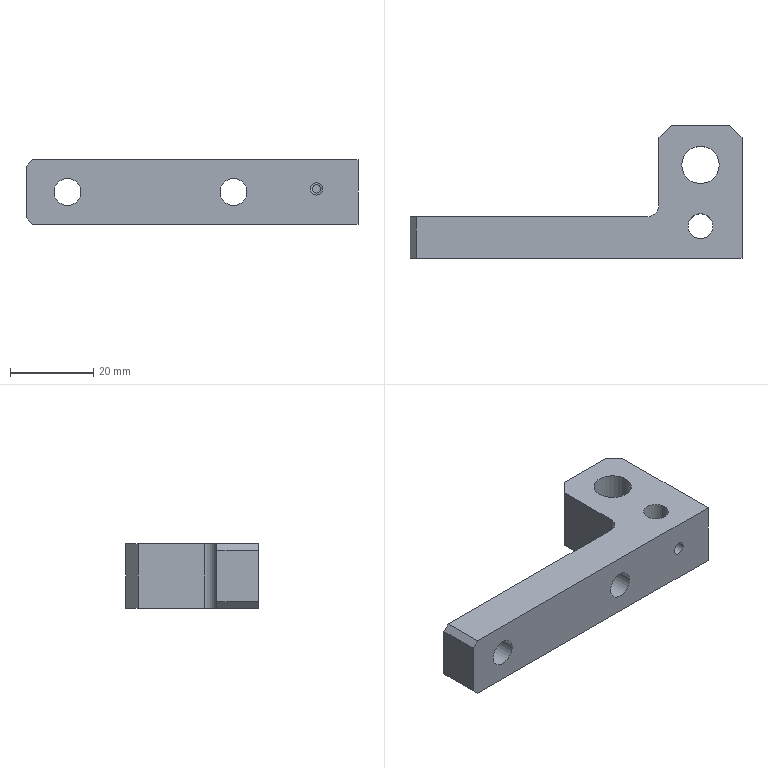NC program | NX | posted with a generic post | part box 80 x 32 x 15.5 mm
Lines 3921 to 4741 of 7013:
(PLANAR_MILL_5 , TOOL : D4-12-D4-50-3T-FINISH)
N7792 T11 M6
N7794 G53
N7796 G17 G0 G90 X26.347 Y-4.914 B0. C0. S3000 M3
N7798 G43 Z20. H11
N7800 Z0.5
N7802 G94 G1 X26.264 Y-5.105 Z0.499 F200.
N7804 X26.137 Y-5.509 Z0.497
N7806 X26.054 Y-5.924 Z0.494
N7808 X26.015 Y-6.345 Z0.492
N7810 Y-6.655 Z0.491
N7812 X26.054 Y-7.076 Z0.488
N7814 X26.137 Y-7.491 Z0.486
N7816 X26.264 Y-7.895 Z0.484
N7818 X26.433 Y-8.283 Z0.482
N7820 X26.641 Y-8.65 Z0.48
N7822 X26.888 Y-8.994 Z0.477
N7824 X27.17 Y-9.31 Z0.475
N7826 X27.484 Y-9.594 Z0.473
N7828 X27.826 Y-9.843 Z0.471
N7830 X28.192 Y-10.055 Z0.468
N7832 X28.579 Y-10.226 Z0.466
N7834 X28.982 Y-10.356 Z0.464
N7836 X29.396 Y-10.442 Z0.462
N7838 X29.817 Y-10.484 Z0.46
N7840 X30.24 Y-10.481 Z0.457
N7842 X30.66 Y-10.433 Z0.455
N7844 X31.073 Y-10.341 Z0.453
N7846 X31.474 Y-10.205 Z0.451
N7848 X31.859 Y-10.028 Z0.449
N7850 X32.126 Y-9.874 Z0.447
N7852 X32.477 Y-9.626 Z0.445
N7854 X32.799 Y-9.341 Z0.442
N7856 X33.088 Y-9.024 Z0.44
N7858 X33.341 Y-8.677 Z0.438
N7860 X33.556 Y-8.305 Z0.436
N7862 X33.73 Y-7.912 Z0.433
N7864 X33.86 Y-7.503 Z0.431
N7866 X33.945 Y-7.082 Z0.429
N7868 X33.985 Y-6.655 Z0.427
N7870 Y-6.345 Z0.425
N7872 X33.945 Y-5.918 Z0.423
N7874 X33.86 Y-5.497 Z0.421
N7876 X33.73 Y-5.088 Z0.418
N7878 X33.556 Y-4.695 Z0.416
N7880 X33.341 Y-4.323 Z0.414
N7882 X33.088 Y-3.976 Z0.412
N7884 X32.799 Y-3.659 Z0.409
N7886 X32.477 Y-3.374 Z0.407
N7888 X32.126 Y-3.126 Z0.405
N7890 X31.859 Y-2.972 Z0.403
N7892 X31.474 Y-2.795 Z0.401
N7894 X31.073 Y-2.659 Z0.399
N7896 X30.66 Y-2.567 Z0.397
N7898 X30.24 Y-2.519 Z0.394
N7900 X29.817 Y-2.516 Z0.392
N7902 X29.396 Y-2.558 Z0.39
N7904 X28.982 Y-2.644 Z0.388
N7906 X28.579 Y-2.774 Z0.385
N7908 X28.192 Y-2.945 Z0.383
N7910 X27.826 Y-3.157 Z0.381
N7912 X27.484 Y-3.406 Z0.379
N7914 X27.17 Y-3.69 Z0.377
N7916 X26.888 Y-4.006 Z0.374
N7918 X26.641 Y-4.35 Z0.372
N7920 X26.433 Y-4.717 Z0.37
N7922 X26.264 Y-5.105 Z0.368
N7924 X26.137 Y-5.509 Z0.366
N7926 X26.054 Y-5.924 Z0.363
N7928 X26.015 Y-6.345 Z0.361
N7930 Y-6.655 Z0.36
N7932 X26.054 Y-7.076 Z0.357
N7934 X26.137 Y-7.491 Z0.355
N7936 X26.264 Y-7.895 Z0.353
N7938 X26.433 Y-8.283 Z0.351
N7940 X26.641 Y-8.65 Z0.348
N7942 X26.888 Y-8.994 Z0.346
N7944 X27.17 Y-9.31 Z0.344
N7946 X27.484 Y-9.594 Z0.342
N7948 X27.826 Y-9.843 Z0.34
N7950 X28.192 Y-10.055 Z0.337
N7952 X28.579 Y-10.226 Z0.335
N7954 X28.982 Y-10.356 Z0.333
N7956 X29.396 Y-10.442 Z0.331
N7958 X29.817 Y-10.484 Z0.328
N7960 X30.24 Y-10.481 Z0.326
N7962 X30.66 Y-10.433 Z0.324
N7964 X31.073 Y-10.341 Z0.322
N7966 X31.474 Y-10.205 Z0.32
N7968 X31.859 Y-10.028 Z0.317
N7970 X32.126 Y-9.874 Z0.316
N7972 X32.477 Y-9.626 Z0.314
N7974 X32.799 Y-9.341 Z0.311
N7976 X33.088 Y-9.024 Z0.309
N7978 X33.341 Y-8.677 Z0.307
N7980 X33.556 Y-8.305 Z0.305
N7982 X33.73 Y-7.912 Z0.302
N7984 X33.86 Y-7.503 Z0.3
N7986 X33.945 Y-7.082 Z0.298
N7988 X33.985 Y-6.655 Z0.296
N7990 Y-6.345 Z0.294
N7992 X33.945 Y-5.918 Z0.292
N7994 X33.86 Y-5.497 Z0.289
N7996 X33.73 Y-5.088 Z0.287
N7998 X33.556 Y-4.695 Z0.285
N8000 X33.341 Y-4.323 Z0.283
N8002 X33.088 Y-3.976 Z0.28
N8004 X32.799 Y-3.659 Z0.278
N8006 X32.477 Y-3.374 Z0.276
N8008 X32.126 Y-3.126 Z0.274
N8010 X31.859 Y-2.972 Z0.272
N8012 X31.474 Y-2.795 Z0.27
N8014 X31.073 Y-2.659 Z0.268
N8016 X30.66 Y-2.567 Z0.265
N8018 X30.24 Y-2.519 Z0.263
N8020 X29.817 Y-2.516 Z0.261
N8022 X29.396 Y-2.558 Z0.259
N8024 X28.982 Y-2.644 Z0.257
N8026 X28.579 Y-2.774 Z0.254
N8028 X28.192 Y-2.945 Z0.252
N8030 X27.826 Y-3.157 Z0.25
N8032 X27.484 Y-3.406 Z0.248
N8034 X27.17 Y-3.69 Z0.245
N8036 X26.888 Y-4.006 Z0.243
N8038 X26.641 Y-4.35 Z0.241
N8040 X26.433 Y-4.717 Z0.239
N8042 X26.264 Y-5.105 Z0.237
N8044 X26.137 Y-5.509 Z0.234
N8046 X26.054 Y-5.924 Z0.232
N8048 X26.015 Y-6.345 Z0.23
N8050 Y-6.655 Z0.228
N8052 X26.054 Y-7.076 Z0.226
N8054 X26.137 Y-7.491 Z0.224
N8056 X26.264 Y-7.895 Z0.222
N8058 X26.433 Y-8.283 Z0.219
N8060 X26.641 Y-8.65 Z0.217
N8062 X26.888 Y-8.994 Z0.215
N8064 X27.17 Y-9.31 Z0.213
N8066 X27.484 Y-9.594 Z0.211
N8068 X27.826 Y-9.843 Z0.208
N8070 X28.192 Y-10.055 Z0.206
N8072 X28.579 Y-10.226 Z0.204
N8074 X28.982 Y-10.356 Z0.202
N8076 X29.396 Y-10.442 Z0.2
N8078 X29.817 Y-10.484 Z0.197
N8080 X30.24 Y-10.481 Z0.195
N8082 X30.66 Y-10.433 Z0.193
N8084 X31.073 Y-10.341 Z0.191
N8086 X31.474 Y-10.205 Z0.188
N8088 X31.859 Y-10.028 Z0.186
N8090 X32.126 Y-9.874 Z0.185
N8092 X32.477 Y-9.626 Z0.182
N8094 X32.799 Y-9.341 Z0.18
N8096 X33.088 Y-9.024 Z0.178
N8098 X33.341 Y-8.677 Z0.176
N8100 X33.556 Y-8.305 Z0.173
N8102 X33.73 Y-7.912 Z0.171
N8104 X33.86 Y-7.503 Z0.169
N8106 X33.945 Y-7.082 Z0.167
N8108 X33.985 Y-6.655 Z0.164
N8110 Y-6.345 Z0.163
N8112 X33.945 Y-5.918 Z0.161
N8114 X33.86 Y-5.497 Z0.158
N8116 X33.73 Y-5.088 Z0.156
N8118 X33.556 Y-4.695 Z0.154
N8120 X33.341 Y-4.323 Z0.152
N8122 X33.088 Y-3.976 Z0.149
N8124 X32.799 Y-3.659 Z0.147
N8126 X32.477 Y-3.374 Z0.145
N8128 X32.126 Y-3.126 Z0.143
N8130 X31.859 Y-2.972 Z0.141
N8132 X31.474 Y-2.795 Z0.139
N8134 X31.073 Y-2.659 Z0.137
N8136 X30.66 Y-2.567 Z0.134
N8138 X30.24 Y-2.519 Z0.132
N8140 X29.817 Y-2.516 Z0.13
N8142 X29.396 Y-2.558 Z0.128
N8144 X28.982 Y-2.644 Z0.125
N8146 X28.579 Y-2.774 Z0.123
N8148 X28.192 Y-2.945 Z0.121
N8150 X27.826 Y-3.157 Z0.119
N8152 X27.484 Y-3.406 Z0.117
N8154 X27.17 Y-3.69 Z0.114
N8156 X26.888 Y-4.006 Z0.112
N8158 X26.641 Y-4.35 Z0.11
N8160 X26.433 Y-4.717 Z0.108
N8162 X26.264 Y-5.105 Z0.105
N8164 X26.137 Y-5.509 Z0.103
N8166 X26.054 Y-5.924 Z0.101
N8168 X26.015 Y-6.345 Z0.099
N8170 Y-6.655 Z0.097
N8172 X26.054 Y-7.076 Z0.095
N8174 X26.137 Y-7.491 Z0.093
N8176 X26.264 Y-7.895 Z0.091
N8178 X26.433 Y-8.283 Z0.088
N8180 X26.641 Y-8.65 Z0.086
N8182 X26.888 Y-8.994 Z0.084
N8184 X27.17 Y-9.31 Z0.082
N8186 X27.484 Y-9.594 Z0.079
N8188 X27.826 Y-9.843 Z0.077
N8190 X28.192 Y-10.055 Z0.075
N8192 X28.579 Y-10.226 Z0.073
N8194 X28.982 Y-10.356 Z0.071
N8196 X29.396 Y-10.442 Z0.068
N8198 X29.817 Y-10.484 Z0.066
N8200 X30.24 Y-10.481 Z0.064
N8202 X30.66 Y-10.433 Z0.062
N8204 X31.073 Y-10.341 Z0.06
N8206 X31.474 Y-10.205 Z0.057
N8208 X31.859 Y-10.028 Z0.055
N8210 X32.126 Y-9.874 Z0.054
N8212 X32.477 Y-9.626 Z0.051
N8214 X32.799 Y-9.341 Z0.049
N8216 X33.088 Y-9.024 Z0.047
N8218 X33.341 Y-8.677 Z0.045
N8220 X33.556 Y-8.305 Z0.042
N8222 X33.73 Y-7.912 Z0.04
N8224 X33.86 Y-7.503 Z0.038
N8226 X33.945 Y-7.082 Z0.036
N8228 X33.985 Y-6.655 Z0.033
N8230 Y-6.345 Z0.032
N8232 X33.945 Y-5.918 Z0.029
N8234 X33.86 Y-5.497 Z0.027
N8236 X33.73 Y-5.088 Z0.025
N8238 X33.556 Y-4.695 Z0.023
N8240 X33.341 Y-4.323 Z0.02
N8242 X33.088 Y-3.976 Z0.018
N8244 X32.799 Y-3.659 Z0.016
N8246 X32.477 Y-3.374 Z0.014
N8248 X32.126 Y-3.126 Z0.011
N8250 X31.859 Y-2.972 Z0.01
N8252 X31.474 Y-2.795 Z0.008
N8254 X31.073 Y-2.659 Z0.005
N8256 X30.66 Y-2.567 Z0.003
N8258 X30.24 Y-2.519 Z0.001
N8260 X29.817 Y-2.516 Z-0.001
N8262 X29.396 Y-2.558 Z-0.004
N8264 X28.982 Y-2.644 Z-0.006
N8266 X28.579 Y-2.774 Z-0.008
N8268 X28.192 Y-2.945 Z-0.01
N8270 X27.826 Y-3.157 Z-0.012
N8272 X27.484 Y-3.406 Z-0.015
N8274 X27.17 Y-3.69 Z-0.017
N8276 X26.888 Y-4.006 Z-0.019
N8278 X26.641 Y-4.35 Z-0.021
N8280 X26.433 Y-4.717 Z-0.023
N8282 X26.264 Y-5.105 Z-0.026
N8284 X26.137 Y-5.509 Z-0.028
N8286 X26.054 Y-5.924 Z-0.03
N8288 X26.015 Y-6.345 Z-0.032
N8290 Y-6.655 Z-0.034
N8292 X26.054 Y-7.076 Z-0.036
N8294 X26.137 Y-7.491 Z-0.038
N8296 X26.264 Y-7.895 Z-0.041
N8298 X26.433 Y-8.283 Z-0.043
N8300 X26.641 Y-8.65 Z-0.045
N8302 X26.888 Y-8.994 Z-0.047
N8304 X27.17 Y-9.31 Z-0.049
N8306 X27.484 Y-9.594 Z-0.052
N8308 X27.826 Y-9.843 Z-0.054
N8310 X28.192 Y-10.055 Z-0.056
N8312 X28.579 Y-10.226 Z-0.058
N8314 X28.982 Y-10.356 Z-0.061
N8316 X29.396 Y-10.442 Z-0.063
N8318 X29.817 Y-10.484 Z-0.065
N8320 X30.24 Y-10.481 Z-0.067
N8322 X30.66 Y-10.433 Z-0.069
N8324 X31.073 Y-10.341 Z-0.072
N8326 X31.474 Y-10.205 Z-0.074
N8328 X31.859 Y-10.028 Z-0.076
N8330 X32.126 Y-9.874 Z-0.078
N8332 X32.477 Y-9.626 Z-0.08
N8334 X32.799 Y-9.341 Z-0.082
N8336 X33.088 Y-9.024 Z-0.084
N8338 X33.341 Y-8.677 Z-0.087
N8340 X33.556 Y-8.305 Z-0.089
N8342 X33.73 Y-7.912 Z-0.091
N8344 X33.86 Y-7.503 Z-0.093
N8346 X33.945 Y-7.082 Z-0.096
N8348 X33.985 Y-6.655 Z-0.098
N8350 Y-6.345 Z-0.099
N8352 X33.945 Y-5.918 Z-0.102
N8354 X33.86 Y-5.497 Z-0.104
N8356 X33.73 Y-5.088 Z-0.106
N8358 X33.556 Y-4.695 Z-0.108
N8360 X33.341 Y-4.323 Z-0.111
N8362 X33.088 Y-3.976 Z-0.113
N8364 X32.799 Y-3.659 Z-0.115
N8366 X32.477 Y-3.374 Z-0.117
N8368 X32.126 Y-3.126 Z-0.12
N8370 X31.859 Y-2.972 Z-0.121
N8372 X31.474 Y-2.795 Z-0.124
N8374 X31.073 Y-2.659 Z-0.126
N8376 X30.66 Y-2.567 Z-0.128
N8378 X30.24 Y-2.519 Z-0.13
N8380 X29.817 Y-2.516 Z-0.132
N8382 X29.396 Y-2.558 Z-0.135
N8384 X28.982 Y-2.644 Z-0.137
N8386 X28.579 Y-2.774 Z-0.139
N8388 X28.192 Y-2.945 Z-0.141
N8390 X27.826 Y-3.157 Z-0.144
N8392 X27.484 Y-3.406 Z-0.146
N8394 X27.17 Y-3.69 Z-0.148
N8396 X26.888 Y-4.006 Z-0.15
N8398 X26.641 Y-4.35 Z-0.152
N8400 X26.433 Y-4.717 Z-0.155
N8402 X26.264 Y-5.105 Z-0.157
N8404 X26.137 Y-5.509 Z-0.159
N8406 X26.054 Y-5.924 Z-0.161
N8408 X26.015 Y-6.345 Z-0.163
N8410 Y-6.655 Z-0.165
N8412 X26.054 Y-7.076 Z-0.167
N8414 X26.137 Y-7.491 Z-0.169
N8416 X26.264 Y-7.895 Z-0.172
N8418 X26.433 Y-8.283 Z-0.174
N8420 X26.641 Y-8.65 Z-0.176
N8422 X26.888 Y-8.994 Z-0.178
N8424 X27.17 Y-9.31 Z-0.181
N8426 X27.484 Y-9.594 Z-0.183
N8428 X27.826 Y-9.843 Z-0.185
N8430 X28.192 Y-10.055 Z-0.187
N8432 X28.579 Y-10.226 Z-0.189
N8434 X28.982 Y-10.356 Z-0.192
N8436 X29.396 Y-10.442 Z-0.194
N8438 X29.817 Y-10.484 Z-0.196
N8440 X30.24 Y-10.481 Z-0.198
N8442 X30.66 Y-10.433 Z-0.201
N8444 X31.073 Y-10.341 Z-0.203
N8446 X31.474 Y-10.205 Z-0.205
N8448 X31.859 Y-10.028 Z-0.207
N8450 X32.126 Y-9.874 Z-0.209
N8452 X32.477 Y-9.626 Z-0.211
N8454 X32.799 Y-9.341 Z-0.213
N8456 X33.088 Y-9.024 Z-0.216
N8458 X33.341 Y-8.677 Z-0.218
N8460 X33.556 Y-8.305 Z-0.22
N8462 X33.73 Y-7.912 Z-0.222
N8464 X33.86 Y-7.503 Z-0.225
N8466 X33.945 Y-7.082 Z-0.227
N8468 X33.985 Y-6.655 Z-0.229
N8470 Y-6.345 Z-0.231
N8472 X33.945 Y-5.918 Z-0.233
N8474 X33.86 Y-5.497 Z-0.235
N8476 X33.73 Y-5.088 Z-0.237
N8478 X33.556 Y-4.695 Z-0.24
N8480 X33.341 Y-4.323 Z-0.242
N8482 X33.088 Y-3.976 Z-0.244
N8484 X32.799 Y-3.659 Z-0.246
N8486 X32.477 Y-3.374 Z-0.249
N8488 X32.126 Y-3.126 Z-0.251
N8490 X31.859 Y-2.972 Z-0.252
N8492 X31.474 Y-2.795 Z-0.255
N8494 X31.073 Y-2.659 Z-0.257
N8496 X30.66 Y-2.567 Z-0.259
N8498 X30.24 Y-2.519 Z-0.261
N8500 X29.817 Y-2.516 Z-0.264
N8502 X29.396 Y-2.558 Z-0.266
N8504 X28.982 Y-2.644 Z-0.268
N8506 X28.579 Y-2.774 Z-0.27
N8508 X28.192 Y-2.945 Z-0.272
N8510 X27.826 Y-3.157 Z-0.275
N8512 X27.484 Y-3.406 Z-0.277
N8514 X27.17 Y-3.69 Z-0.279
N8516 X26.888 Y-4.006 Z-0.281
N8518 X26.641 Y-4.35 Z-0.284
N8520 X26.433 Y-4.717 Z-0.286
N8522 X26.264 Y-5.105 Z-0.288
N8524 X26.137 Y-5.509 Z-0.29
N8526 X26.054 Y-5.924 Z-0.292
N8528 X26.015 Y-6.345 Z-0.295
N8530 Y-6.655 Z-0.296
N8532 X26.054 Y-7.076 Z-0.298
N8534 X26.137 Y-7.491 Z-0.301
N8536 X26.264 Y-7.895 Z-0.303
N8538 X26.433 Y-8.283 Z-0.305
N8540 X26.641 Y-8.65 Z-0.307
N8542 X26.888 Y-8.994 Z-0.309
N8544 X27.17 Y-9.31 Z-0.312
N8546 X27.484 Y-9.594 Z-0.314
N8548 X27.826 Y-9.843 Z-0.316
N8550 X28.192 Y-10.055 Z-0.318
N8552 X28.579 Y-10.226 Z-0.321
N8554 X28.982 Y-10.356 Z-0.323
N8556 X29.396 Y-10.442 Z-0.325
N8558 X29.817 Y-10.484 Z-0.327
N8560 X30.24 Y-10.481 Z-0.329
N8562 X30.66 Y-10.433 Z-0.332
N8564 X31.073 Y-10.341 Z-0.334
N8566 X31.474 Y-10.205 Z-0.336
N8568 X31.859 Y-10.028 Z-0.338
N8570 X32.126 Y-9.874 Z-0.34
N8572 X32.477 Y-9.626 Z-0.342
N8574 X32.799 Y-9.341 Z-0.344
N8576 X33.088 Y-9.024 Z-0.347
N8578 X33.341 Y-8.677 Z-0.349
N8580 X33.556 Y-8.305 Z-0.351
N8582 X33.73 Y-7.912 Z-0.353
N8584 X33.86 Y-7.503 Z-0.356
N8586 X33.945 Y-7.082 Z-0.358
N8588 X33.985 Y-6.655 Z-0.36
N8590 Y-6.345 Z-0.362
N8592 X33.945 Y-5.918 Z-0.364
N8594 X33.86 Y-5.497 Z-0.366
N8596 X33.73 Y-5.088 Z-0.369
N8598 X33.556 Y-4.695 Z-0.371
N8600 X33.341 Y-4.323 Z-0.373
N8602 X33.088 Y-3.976 Z-0.375
N8604 X32.799 Y-3.659 Z-0.378
N8606 X32.477 Y-3.374 Z-0.38
N8608 X32.126 Y-3.126 Z-0.382
N8610 X31.859 Y-2.972 Z-0.384
N8612 X31.474 Y-2.795 Z-0.386
N8614 X31.073 Y-2.659 Z-0.388
N8616 X30.66 Y-2.567 Z-0.39
N8618 X30.24 Y-2.519 Z-0.392
N8620 X29.817 Y-2.516 Z-0.395
N8622 X29.396 Y-2.558 Z-0.397
N8624 X28.982 Y-2.644 Z-0.399
N8626 X28.579 Y-2.774 Z-0.401
N8628 X28.192 Y-2.945 Z-0.404
N8630 X27.826 Y-3.157 Z-0.406
N8632 X27.484 Y-3.406 Z-0.408
N8634 X27.17 Y-3.69 Z-0.41
N8636 X26.888 Y-4.006 Z-0.412
N8638 X26.641 Y-4.35 Z-0.415
N8640 X26.433 Y-4.717 Z-0.417
N8642 X26.264 Y-5.105 Z-0.419
N8644 X26.137 Y-5.509 Z-0.421
N8646 X26.054 Y-5.924 Z-0.424
N8648 X26.015 Y-6.345 Z-0.426
N8650 Y-6.655 Z-0.427
N8652 X26.054 Y-7.076 Z-0.43
N8654 X26.137 Y-7.491 Z-0.432
N8656 X26.264 Y-7.895 Z-0.434
N8658 X26.433 Y-8.283 Z-0.436
N8660 X26.641 Y-8.65 Z-0.438
N8662 X26.888 Y-8.994 Z-0.441
N8664 X27.17 Y-9.31 Z-0.443
N8666 X27.484 Y-9.594 Z-0.445
N8668 X27.826 Y-9.843 Z-0.447
N8670 X28.192 Y-10.055 Z-0.449
N8672 X28.579 Y-10.226 Z-0.452
N8674 X28.982 Y-10.356 Z-0.454
N8676 X29.396 Y-10.442 Z-0.456
N8678 X29.817 Y-10.484 Z-0.458
N8680 X30.24 Y-10.481 Z-0.461
N8682 X30.66 Y-10.433 Z-0.463
N8684 X31.073 Y-10.341 Z-0.465
N8686 X31.474 Y-10.205 Z-0.467
N8688 X31.859 Y-10.028 Z-0.469
N8690 X32.126 Y-9.874 Z-0.471
N8692 X32.477 Y-9.626 Z-0.473
N8694 X32.799 Y-9.341 Z-0.476
N8696 X33.088 Y-9.024 Z-0.478
N8698 X33.341 Y-8.677 Z-0.48
N8700 X33.556 Y-8.305 Z-0.482
N8702 X33.73 Y-7.912 Z-0.485
N8704 X33.86 Y-7.503 Z-0.487
N8706 X33.945 Y-7.082 Z-0.489
N8708 X33.985 Y-6.655 Z-0.491
N8710 Y-6.345 Z-0.493
N8712 X33.945 Y-5.918 Z-0.495
N8714 X33.86 Y-5.497 Z-0.497
N8716 X33.73 Y-5.088 Z-0.5
N8718 X33.556 Y-4.695 Z-0.502
N8720 X33.341 Y-4.323 Z-0.504
N8722 X33.088 Y-3.976 Z-0.506
N8724 X32.799 Y-3.659 Z-0.509
N8726 X32.477 Y-3.374 Z-0.511
N8728 X32.126 Y-3.126 Z-0.513
N8730 X31.859 Y-2.972 Z-0.515
N8732 X31.474 Y-2.795 Z-0.517
N8734 X31.073 Y-2.659 Z-0.519
N8736 X30.66 Y-2.567 Z-0.521
N8738 X30.24 Y-2.519 Z-0.524
N8740 X29.817 Y-2.516 Z-0.526
N8742 X29.396 Y-2.558 Z-0.528
N8744 X28.982 Y-2.644 Z-0.53
N8746 X28.579 Y-2.774 Z-0.532
N8748 X28.192 Y-2.945 Z-0.535
N8750 X27.826 Y-3.157 Z-0.537
N8752 X27.484 Y-3.406 Z-0.539
N8754 X27.17 Y-3.69 Z-0.541
N8756 X26.888 Y-4.006 Z-0.544
N8758 X26.641 Y-4.35 Z-0.546
N8760 X26.433 Y-4.717 Z-0.548
N8762 X26.264 Y-5.105 Z-0.55
N8764 X26.137 Y-5.509 Z-0.552
N8766 X26.054 Y-5.924 Z-0.555
N8768 X26.015 Y-6.345 Z-0.557
N8770 Y-6.655 Z-0.558
N8772 X26.054 Y-7.076 Z-0.561
N8774 X26.137 Y-7.491 Z-0.563
N8776 X26.264 Y-7.895 Z-0.565
N8778 X26.433 Y-8.283 Z-0.567
N8780 X26.641 Y-8.65 Z-0.57
N8782 X26.888 Y-8.994 Z-0.572
N8784 X27.17 Y-9.31 Z-0.574
N8786 X27.484 Y-9.594 Z-0.576
N8788 X27.826 Y-9.843 Z-0.578
N8790 X28.192 Y-10.055 Z-0.581
N8792 X28.579 Y-10.226 Z-0.583
N8794 X28.982 Y-10.356 Z-0.585
N8796 X29.396 Y-10.442 Z-0.587
N8798 X29.817 Y-10.484 Z-0.59
N8800 X30.24 Y-10.481 Z-0.592
N8802 X30.66 Y-10.433 Z-0.594
N8804 X31.073 Y-10.341 Z-0.596
N8806 X31.474 Y-10.205 Z-0.598
N8808 X31.859 Y-10.028 Z-0.601
N8810 X32.126 Y-9.874 Z-0.602
N8812 X32.477 Y-9.626 Z-0.604
N8814 X32.799 Y-9.341 Z-0.607
N8816 X33.088 Y-9.024 Z-0.609
N8818 X33.341 Y-8.677 Z-0.611
N8820 X33.556 Y-8.305 Z-0.613
N8822 X33.73 Y-7.912 Z-0.616
N8824 X33.86 Y-7.503 Z-0.618
N8826 X33.945 Y-7.082 Z-0.62
N8828 X33.985 Y-6.655 Z-0.622
N8830 Y-6.345 Z-0.624
N8832 X33.945 Y-5.918 Z-0.626
N8834 X33.86 Y-5.497 Z-0.629
N8836 X33.73 Y-5.088 Z-0.631
N8838 X33.556 Y-4.695 Z-0.633
N8840 X33.341 Y-4.323 Z-0.635
N8842 X33.088 Y-3.976 Z-0.638
N8844 X32.799 Y-3.659 Z-0.64
N8846 X32.477 Y-3.374 Z-0.642
N8848 X32.126 Y-3.126 Z-0.644
N8850 X31.859 Y-2.972 Z-0.646
N8852 X31.474 Y-2.795 Z-0.648
N8854 X31.073 Y-2.659 Z-0.65
N8856 X30.66 Y-2.567 Z-0.653
N8858 X30.24 Y-2.519 Z-0.655
N8860 X29.817 Y-2.516 Z-0.657
N8862 X29.396 Y-2.558 Z-0.659
N8864 X28.982 Y-2.644 Z-0.661
N8866 X28.579 Y-2.774 Z-0.664
N8868 X28.192 Y-2.945 Z-0.666
N8870 X27.826 Y-3.157 Z-0.668
N8872 X27.484 Y-3.406 Z-0.67
N8874 X27.17 Y-3.69 Z-0.672
N8876 X26.888 Y-4.006 Z-0.675
N8878 X26.641 Y-4.35 Z-0.677
N8880 X26.433 Y-4.717 Z-0.679
N8882 X26.264 Y-5.105 Z-0.681
N8884 X26.137 Y-5.509 Z-0.684
N8886 X26.054 Y-5.924 Z-0.686
N8888 X26.015 Y-6.345 Z-0.688
N8890 Y-6.655 Z-0.69
N8892 X26.054 Y-7.076 Z-0.692
N8894 X26.137 Y-7.491 Z-0.694
N8896 X26.264 Y-7.895 Z-0.696
N8898 X26.433 Y-8.283 Z-0.698
N8900 X26.641 Y-8.65 Z-0.701
N8902 X26.888 Y-8.994 Z-0.703
N8904 X27.17 Y-9.31 Z-0.705
N8906 X27.484 Y-9.594 Z-0.707
N8908 X27.826 Y-9.843 Z-0.71
N8910 X28.192 Y-10.055 Z-0.712
N8912 X28.579 Y-10.226 Z-0.714
N8914 X28.982 Y-10.356 Z-0.716
N8916 X29.396 Y-10.442 Z-0.718
N8918 X29.817 Y-10.484 Z-0.721
N8920 X30.24 Y-10.481 Z-0.723
N8922 X30.66 Y-10.433 Z-0.725
N8924 X31.073 Y-10.341 Z-0.727
N8926 X31.474 Y-10.205 Z-0.73
N8928 X31.859 Y-10.028 Z-0.732
N8930 X32.126 Y-9.874 Z-0.733
N8932 X32.477 Y-9.626 Z-0.736
N8934 X32.799 Y-9.341 Z-0.738
N8936 X33.088 Y-9.024 Z-0.74
N8938 X33.341 Y-8.677 Z-0.742
N8940 X33.556 Y-8.305 Z-0.745
N8942 X33.73 Y-7.912 Z-0.747
N8944 X33.86 Y-7.503 Z-0.749
N8946 X33.945 Y-7.082 Z-0.751
N8948 X33.985 Y-6.655 Z-0.754
N8950 Y-6.345 Z-0.755
N8952 X33.945 Y-5.918 Z-0.757
N8954 X33.86 Y-5.497 Z-0.76
N8956 X33.73 Y-5.088 Z-0.762
N8958 X33.556 Y-4.695 Z-0.764
N8960 X33.341 Y-4.323 Z-0.766
N8962 X33.088 Y-3.976 Z-0.769
N8964 X32.799 Y-3.659 Z-0.771
N8966 X32.477 Y-3.374 Z-0.773
N8968 X32.126 Y-3.126 Z-0.775
N8970 X31.859 Y-2.972 Z-0.777
N8972 X31.474 Y-2.795 Z-0.779
N8974 X31.073 Y-2.659 Z-0.781
N8976 X30.66 Y-2.567 Z-0.784
N8978 X30.24 Y-2.519 Z-0.786
N8980 X29.817 Y-2.516 Z-0.788
N8982 X29.396 Y-2.558 Z-0.79
N8984 X28.982 Y-2.644 Z-0.793
N8986 X28.579 Y-2.774 Z-0.795
N8988 X28.192 Y-2.945 Z-0.797
N8990 X27.826 Y-3.157 Z-0.799
N8992 X27.484 Y-3.406 Z-0.801
N8994 X27.17 Y-3.69 Z-0.804
N8996 X26.888 Y-4.006 Z-0.806
N8998 X26.641 Y-4.35 Z-0.808
N9000 X26.433 Y-4.717 Z-0.81
N9002 X26.264 Y-5.105 Z-0.812
N9004 X26.137 Y-5.509 Z-0.815
N9006 X26.054 Y-5.924 Z-0.817
N9008 X26.015 Y-6.345 Z-0.819
N9010 Y-6.655 Z-0.821
N9012 X26.054 Y-7.076 Z-0.823
N9014 X26.137 Y-7.491 Z-0.825
N9016 X26.264 Y-7.895 Z-0.827
N9018 X26.433 Y-8.283 Z-0.83
N9020 X26.641 Y-8.65 Z-0.832
N9022 X26.888 Y-8.994 Z-0.834
N9024 X27.17 Y-9.31 Z-0.836
N9026 X27.484 Y-9.594 Z-0.838
N9028 X27.826 Y-9.843 Z-0.841
N9030 X28.192 Y-10.055 Z-0.843
N9032 X28.579 Y-10.226 Z-0.845
N9034 X28.982 Y-10.356 Z-0.847
N9036 X29.396 Y-10.442 Z-0.85
N9038 X29.817 Y-10.484 Z-0.852
N9040 X30.24 Y-10.481 Z-0.854
N9042 X30.66 Y-10.433 Z-0.856
N9044 X31.073 Y-10.341 Z-0.858
N9046 X31.474 Y-10.205 Z-0.861
N9048 X31.859 Y-10.028 Z-0.863
N9050 X32.126 Y-9.874 Z-0.864
N9052 X32.477 Y-9.626 Z-0.867
N9054 X32.799 Y-9.341 Z-0.869
N9056 X33.088 Y-9.024 Z-0.871
N9058 X33.341 Y-8.677 Z-0.873
N9060 X33.556 Y-8.305 Z-0.876
N9062 X33.73 Y-7.912 Z-0.878
N9064 X33.86 Y-7.503 Z-0.88
N9066 X33.945 Y-7.082 Z-0.882
N9068 X33.985 Y-6.655 Z-0.885
N9070 Y-6.345 Z-0.886
N9072 X33.945 Y-5.918 Z-0.889
N9074 X33.86 Y-5.497 Z-0.891
N9076 X33.73 Y-5.088 Z-0.893
N9078 X33.556 Y-4.695 Z-0.895
N9080 X33.341 Y-4.323 Z-0.898
N9082 X33.088 Y-3.976 Z-0.9
N9084 X32.799 Y-3.659 Z-0.902
N9086 X32.477 Y-3.374 Z-0.904
N9088 X32.126 Y-3.126 Z-0.907
N9090 X31.859 Y-2.972 Z-0.908
N9092 X31.474 Y-2.795 Z-0.91
N9094 X31.073 Y-2.659 Z-0.913
N9096 X30.66 Y-2.567 Z-0.915
N9098 X30.24 Y-2.519 Z-0.917
N9100 X29.817 Y-2.516 Z-0.919
N9102 X29.396 Y-2.558 Z-0.921
N9104 X28.982 Y-2.644 Z-0.924
N9106 X28.579 Y-2.774 Z-0.926
N9108 X28.192 Y-2.945 Z-0.928
N9110 X27.826 Y-3.157 Z-0.93
N9112 X27.484 Y-3.406 Z-0.933
N9114 X27.17 Y-3.69 Z-0.935
N9116 X26.888 Y-4.006 Z-0.937
N9118 X26.641 Y-4.35 Z-0.939
N9120 X26.433 Y-4.717 Z-0.941
N9122 X26.264 Y-5.105 Z-0.944
N9124 X26.137 Y-5.509 Z-0.946
N9126 X26.054 Y-5.924 Z-0.948
N9128 X26.015 Y-6.345 Z-0.95
N9130 Y-6.655 Z-0.952
N9132 X26.054 Y-7.076 Z-0.954
N9134 X26.137 Y-7.491 Z-0.956
N9136 X26.264 Y-7.895 Z-0.959
N9138 X26.433 Y-8.283 Z-0.961
N9140 X26.641 Y-8.65 Z-0.963
N9142 X26.888 Y-8.994 Z-0.965
N9144 X27.17 Y-9.31 Z-0.967
N9146 X27.484 Y-9.594 Z-0.97
N9148 X27.826 Y-9.843 Z-0.972
N9150 X28.192 Y-10.055 Z-0.974
N9152 X28.579 Y-10.226 Z-0.976
N9154 X28.982 Y-10.356 Z-0.978
N9156 X29.396 Y-10.442 Z-0.981
N9158 X29.817 Y-10.484 Z-0.983
N9160 X30.24 Y-10.481 Z-0.985
N9162 X30.66 Y-10.433 Z-0.987
N9164 X31.073 Y-10.341 Z-0.99
N9166 X31.474 Y-10.205 Z-0.992
N9168 X31.859 Y-10.028 Z-0.994
N9170 X32.126 Y-9.874 Z-0.996
N9172 X32.477 Y-9.626 Z-0.998
N9174 X32.799 Y-9.341 Z-1.
N9176 X33.088 Y-9.024 Z-1.002
N9178 X33.341 Y-8.677 Z-1.005
N9180 X33.556 Y-8.305 Z-1.007
N9182 X33.73 Y-7.912 Z-1.009
N9184 X33.86 Y-7.503 Z-1.011
N9186 X33.945 Y-7.082 Z-1.014
N9188 X33.985 Y-6.655 Z-1.016
N9190 Y-6.345 Z-1.017
N9192 X33.945 Y-5.918 Z-1.02
N9194 X33.86 Y-5.497 Z-1.022
N9196 X33.73 Y-5.088 Z-1.024
N9198 X33.556 Y-4.695 Z-1.026
N9200 X33.341 Y-4.323 Z-1.029
N9202 X33.088 Y-3.976 Z-1.031
N9204 X32.799 Y-3.659 Z-1.033
N9206 X32.477 Y-3.374 Z-1.035
N9208 X32.126 Y-3.126 Z-1.038
N9210 X31.859 Y-2.972 Z-1.039
N9212 X31.474 Y-2.795 Z-1.042
N9214 X31.073 Y-2.659 Z-1.044
N9216 X30.66 Y-2.567 Z-1.046
N9218 X30.24 Y-2.519 Z-1.048
N9220 X29.817 Y-2.516 Z-1.05
N9222 X29.396 Y-2.558 Z-1.053
N9224 X28.982 Y-2.644 Z-1.055
N9226 X28.579 Y-2.774 Z-1.057
N9228 X28.192 Y-2.945 Z-1.059
N9230 X27.826 Y-3.157 Z-1.061
N9232 X27.484 Y-3.406 Z-1.064
N9234 X27.17 Y-3.69 Z-1.066
N9236 X26.888 Y-4.006 Z-1.068
N9238 X26.641 Y-4.35 Z-1.07
N9240 X26.433 Y-4.717 Z-1.073
N9242 X26.264 Y-5.105 Z-1.075
N9244 X26.137 Y-5.509 Z-1.077
N9246 X26.054 Y-5.924 Z-1.079
N9248 X26.015 Y-6.345 Z-1.081
N9250 Y-6.655 Z-1.083
N9252 X26.054 Y-7.076 Z-1.085
N9254 X26.137 Y-7.491 Z-1.087
N9256 X26.264 Y-7.895 Z-1.09
N9258 X26.433 Y-8.283 Z-1.092
N9260 X26.641 Y-8.65 Z-1.094
N9262 X26.888 Y-8.994 Z-1.096
N9264 X27.17 Y-9.31 Z-1.099
N9266 X27.484 Y-9.594 Z-1.101
N9268 X27.826 Y-9.843 Z-1.103
N9270 X28.192 Y-10.055 Z-1.105
N9272 X28.579 Y-10.226 Z-1.107
N9274 X28.982 Y-10.356 Z-1.11
N9276 X29.396 Y-10.442 Z-1.112
N9278 X29.817 Y-10.484 Z-1.114
N9280 X30.24 Y-10.481 Z-1.116
N9282 X30.66 Y-10.433 Z-1.118
N9284 X31.073 Y-10.341 Z-1.121
N9286 X31.474 Y-10.205 Z-1.123
N9288 X31.859 Y-10.028 Z-1.125
N9290 X32.126 Y-9.874 Z-1.127
N9292 X32.477 Y-9.626 Z-1.129
N9294 X32.799 Y-9.341 Z-1.131
N9296 X33.088 Y-9.024 Z-1.134
N9298 X33.341 Y-8.677 Z-1.136
N9300 X33.556 Y-8.305 Z-1.138
N9302 X33.73 Y-7.912 Z-1.14
N9304 X33.86 Y-7.503 Z-1.142
N9306 X33.945 Y-7.082 Z-1.145
N9308 X33.985 Y-6.655 Z-1.147
N9310 Y-6.345 Z-1.149
N9312 X33.945 Y-5.918 Z-1.151
N9314 X33.86 Y-5.497 Z-1.153
N9316 X33.73 Y-5.088 Z-1.155
N9318 X33.556 Y-4.695 Z-1.158
N9320 X33.341 Y-4.323 Z-1.16
N9322 X33.088 Y-3.976 Z-1.162
N9324 X32.799 Y-3.659 Z-1.164
N9326 X32.477 Y-3.374 Z-1.167
N9328 X32.126 Y-3.126 Z-1.169
N9330 X31.859 Y-2.972 Z-1.17
N9332 X31.474 Y-2.795 Z-1.173
N9334 X31.073 Y-2.659 Z-1.175
N9336 X30.66 Y-2.567 Z-1.177
N9338 X30.24 Y-2.519 Z-1.179
N9340 X29.817 Y-2.516 Z-1.182
N9342 X29.396 Y-2.558 Z-1.184
N9344 X28.982 Y-2.644 Z-1.186
N9346 X28.579 Y-2.774 Z-1.188
N9348 X28.192 Y-2.945 Z-1.19
N9350 X27.826 Y-3.157 Z-1.193
N9352 X27.484 Y-3.406 Z-1.195
N9354 X27.17 Y-3.69 Z-1.197
N9356 X26.888 Y-4.006 Z-1.199
N9358 X26.641 Y-4.35 Z-1.201
N9360 X26.433 Y-4.717 Z-1.204
N9362 X26.264 Y-5.105 Z-1.206
N9364 X26.137 Y-5.509 Z-1.208
N9366 X26.054 Y-5.924 Z-1.21
N9368 X26.015 Y-6.345 Z-1.213
N9370 Y-6.655 Z-1.214
N9372 X26.054 Y-7.076 Z-1.216
N9374 X26.137 Y-7.491 Z-1.219
N9376 X26.264 Y-7.895 Z-1.221
N9378 X26.433 Y-8.283 Z-1.223
N9380 X26.641 Y-8.65 Z-1.225
N9382 X26.888 Y-8.994 Z-1.227
N9384 X27.17 Y-9.31 Z-1.23
N9386 X27.484 Y-9.594 Z-1.232
N9388 X27.826 Y-9.843 Z-1.234
N9390 X28.192 Y-10.055 Z-1.236
N9392 X28.579 Y-10.226 Z-1.239
N9394 X28.982 Y-10.356 Z-1.241
N9396 X29.396 Y-10.442 Z-1.243
N9398 X29.817 Y-10.484 Z-1.245
N9400 X30.24 Y-10.481 Z-1.247
N9402 X30.66 Y-10.433 Z-1.25
N9404 X31.073 Y-10.341 Z-1.252
N9406 X31.474 Y-10.205 Z-1.254
N9408 X31.859 Y-10.028 Z-1.256
N9410 X32.126 Y-9.874 Z-1.258
N9412 X32.477 Y-9.626 Z-1.26
N9414 X32.799 Y-9.341 Z-1.262
N9416 X33.088 Y-9.024 Z-1.265
N9418 X33.341 Y-8.677 Z-1.267
N9420 X33.556 Y-8.305 Z-1.269
N9422 X33.73 Y-7.912 Z-1.271
N9424 X33.86 Y-7.503 Z-1.274
N9426 X33.945 Y-7.082 Z-1.276